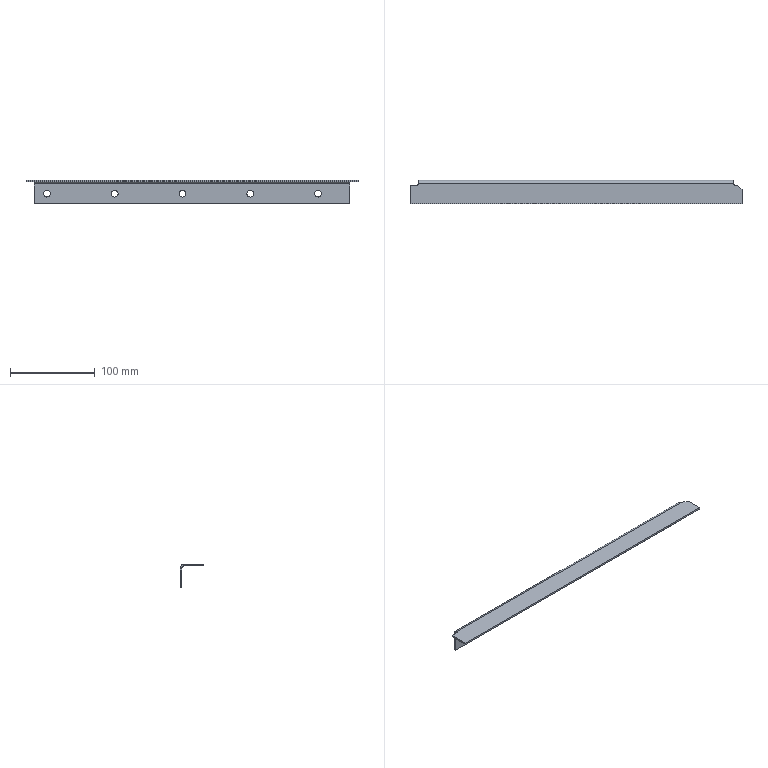Part | SolidWorks | features ICE 2, Chamfer 1, Fillet 1, FlatPattern 1, SMBaseFlange 1, SheetMetal 1 | 1 solid | 29 faces | box 391.9 x 28 x 28 mm | volume 39440 mm3 | plane 15 | cylinder 14 | commonest cylinder face diameters 8 x10 4 x2 5 x1 9 x1
STEP:
#1=CARTESIAN_POINT('',(-171.25,-2.,8.));
#2=VERTEX_POINT('',#1);
#3=CARTESIAN_POINT('',(-171.25,-2.,16.));
#4=VERTEX_POINT('',#3);
#5=CARTESIAN_POINT('',(-171.25,-2.,12.));
#6=DIRECTION('',(0.,1.,0.));
#7=DIRECTION('',(0.,0.,-1.));
#8=AXIS2_PLACEMENT_3D('',#5,#6,#7);
#9=CIRCLE('',#8,4.);
#10=EDGE_CURVE('',#2,#4,#9,.T.);
#11=ORIENTED_EDGE('',*,*,#10,.F.);
#12=CARTESIAN_POINT('',(-171.25,0.,8.));
#13=VERTEX_POINT('',#12);
#14=CARTESIAN_POINT('',(-171.25,-28.001,8.));
#15=DIRECTION('',(0.,1.,0.));
#16=VECTOR('',#15,1000.);
#17=LINE('',#14,#16);
#18=EDGE_CURVE('',#2,#13,#17,.T.);
#19=ORIENTED_EDGE('',*,*,#18,.T.);
#20=CARTESIAN_POINT('',(-171.25,0.,16.));
#21=VERTEX_POINT('',#20);
#22=CARTESIAN_POINT('',(-171.25,0.,12.));
#23=DIRECTION('',(0.,1.,0.));
#24=DIRECTION('',(0.,0.,1.));
#25=AXIS2_PLACEMENT_3D('',#22,#23,#24);
#26=CIRCLE('',#25,4.);
#27=EDGE_CURVE('',#13,#21,#26,.T.);
#28=ORIENTED_EDGE('',*,*,#27,.T.);
#29=CARTESIAN_POINT('',(-171.25,-28.001,16.));
#30=DIRECTION('',(0.,1.,0.));
#31=VECTOR('',#30,1000.);
#32=LINE('',#29,#31);
#33=EDGE_CURVE('',#4,#21,#32,.T.);
#34=ORIENTED_EDGE('',*,*,#33,.F.);
#35=EDGE_LOOP('',(#11,#19,#28,#34));
#36=FACE_OUTER_BOUND('',#35,.T.);
#37=CARTESIAN_POINT('',(-171.25,-28.001,12.));
#38=DIRECTION('',(0.,1.,0.));
#39=DIRECTION('',(0.,0.,1.));
#40=AXIS2_PLACEMENT_3D('',#37,#38,#39);
#41=CYLINDRICAL_SURFACE('',#40,4.);
#42=ADVANCED_FACE('',(#36),#41,.F.);
#43=CARTESIAN_POINT('',(-91.25,-2.,8.));
#44=VERTEX_POINT('',#43);
#45=CARTESIAN_POINT('',(-91.25,-2.,16.));
#46=VERTEX_POINT('',#45);
#47=CARTESIAN_POINT('',(-91.25,-2.,12.));
#48=DIRECTION('',(0.,1.,0.));
#49=DIRECTION('',(0.,0.,-1.));
#50=AXIS2_PLACEMENT_3D('',#47,#48,#49);
#51=CIRCLE('',#50,4.);
#52=EDGE_CURVE('',#44,#46,#51,.T.);
#53=ORIENTED_EDGE('',*,*,#52,.F.);
#54=CARTESIAN_POINT('',(-91.25,0.,8.));
#55=VERTEX_POINT('',#54);
#56=CARTESIAN_POINT('',(-91.25,-28.001,8.));
#57=DIRECTION('',(0.,1.,0.));
#58=VECTOR('',#57,1000.);
#59=LINE('',#56,#58);
#60=EDGE_CURVE('',#44,#55,#59,.T.);
#61=ORIENTED_EDGE('',*,*,#60,.T.);
#62=CARTESIAN_POINT('',(-91.25,0.,16.));
#63=VERTEX_POINT('',#62);
#64=CARTESIAN_POINT('',(-91.25,0.,12.));
#65=DIRECTION('',(0.,1.,0.));
#66=DIRECTION('',(0.,0.,1.));
#67=AXIS2_PLACEMENT_3D('',#64,#65,#66);
#68=CIRCLE('',#67,4.);
#69=EDGE_CURVE('',#55,#63,#68,.T.);
#70=ORIENTED_EDGE('',*,*,#69,.T.);
#71=CARTESIAN_POINT('',(-91.25,-28.001,16.));
#72=DIRECTION('',(0.,1.,0.));
#73=VECTOR('',#72,1000.);
#74=LINE('',#71,#73);
#75=EDGE_CURVE('',#46,#63,#74,.T.);
#76=ORIENTED_EDGE('',*,*,#75,.F.);
#77=EDGE_LOOP('',(#53,#61,#70,#76));
#78=FACE_OUTER_BOUND('',#77,.T.);
#79=CARTESIAN_POINT('',(-91.25,-28.001,12.));
#80=DIRECTION('',(0.,1.,0.));
#81=DIRECTION('',(0.,0.,1.));
#82=AXIS2_PLACEMENT_3D('',#79,#80,#81);
#83=CYLINDRICAL_SURFACE('',#82,4.);
#84=ADVANCED_FACE('',(#78),#83,.F.);
#85=CARTESIAN_POINT('',(-11.25,-2.,8.));
#86=VERTEX_POINT('',#85);
#87=CARTESIAN_POINT('',(-11.25,-2.,16.));
#88=VERTEX_POINT('',#87);
#89=CARTESIAN_POINT('',(-11.25,-2.,12.));
#90=DIRECTION('',(0.,1.,0.));
#91=DIRECTION('',(0.,0.,-1.));
#92=AXIS2_PLACEMENT_3D('',#89,#90,#91);
#93=CIRCLE('',#92,4.);
#94=EDGE_CURVE('',#86,#88,#93,.T.);
#95=ORIENTED_EDGE('',*,*,#94,.F.);
#96=CARTESIAN_POINT('',(-11.25,0.,8.));
#97=VERTEX_POINT('',#96);
#98=CARTESIAN_POINT('',(-11.25,-28.001,8.));
#99=DIRECTION('',(0.,1.,0.));
#100=VECTOR('',#99,1000.);
#101=LINE('',#98,#100);
#102=EDGE_CURVE('',#86,#97,#101,.T.);
#103=ORIENTED_EDGE('',*,*,#102,.T.);
#104=CARTESIAN_POINT('',(-11.25,0.,16.));
#105=VERTEX_POINT('',#104);
#106=CARTESIAN_POINT('',(-11.25,0.,12.));
#107=DIRECTION('',(0.,1.,0.));
#108=DIRECTION('',(0.,0.,1.));
#109=AXIS2_PLACEMENT_3D('',#106,#107,#108);
#110=CIRCLE('',#109,4.);
#111=EDGE_CURVE('',#97,#105,#110,.T.);
#112=ORIENTED_EDGE('',*,*,#111,.T.);
#113=CARTESIAN_POINT('',(-11.25,-28.001,16.));
#114=DIRECTION('',(0.,1.,0.));
#115=VECTOR('',#114,1000.);
#116=LINE('',#113,#115);
#117=EDGE_CURVE('',#88,#105,#116,.T.);
#118=ORIENTED_EDGE('',*,*,#117,.F.);
#119=EDGE_LOOP('',(#95,#103,#112,#118));
#120=FACE_OUTER_BOUND('',#119,.T.);
#121=CARTESIAN_POINT('',(-11.25,-28.001,12.));
#122=DIRECTION('',(0.,1.,0.));
#123=DIRECTION('',(0.,0.,1.));
#124=AXIS2_PLACEMENT_3D('',#121,#122,#123);
#125=CYLINDRICAL_SURFACE('',#124,4.);
#126=ADVANCED_FACE('',(#120),#125,.F.);
#127=CARTESIAN_POINT('',(68.75,-2.,8.));
#128=VERTEX_POINT('',#127);
#129=CARTESIAN_POINT('',(68.75,-2.,16.));
#130=VERTEX_POINT('',#129);
#131=CARTESIAN_POINT('',(68.75,-2.,12.));
#132=DIRECTION('',(0.,1.,0.));
#133=DIRECTION('',(0.,0.,-1.));
#134=AXIS2_PLACEMENT_3D('',#131,#132,#133);
#135=CIRCLE('',#134,4.);
#136=EDGE_CURVE('',#128,#130,#135,.T.);
#137=ORIENTED_EDGE('',*,*,#136,.F.);
#138=CARTESIAN_POINT('',(68.75,0.,8.));
#139=VERTEX_POINT('',#138);
#140=CARTESIAN_POINT('',(68.75,-28.001,8.));
#141=DIRECTION('',(0.,1.,0.));
#142=VECTOR('',#141,1000.);
#143=LINE('',#140,#142);
#144=EDGE_CURVE('',#128,#139,#143,.T.);
#145=ORIENTED_EDGE('',*,*,#144,.T.);
#146=CARTESIAN_POINT('',(68.75,0.,16.));
#147=VERTEX_POINT('',#146);
#148=CARTESIAN_POINT('',(68.75,0.,12.));
#149=DIRECTION('',(0.,1.,0.));
#150=DIRECTION('',(0.,0.,1.));
#151=AXIS2_PLACEMENT_3D('',#148,#149,#150);
#152=CIRCLE('',#151,4.);
#153=EDGE_CURVE('',#139,#147,#152,.T.);
#154=ORIENTED_EDGE('',*,*,#153,.T.);
#155=CARTESIAN_POINT('',(68.75,-28.001,16.));
#156=DIRECTION('',(0.,1.,0.));
#157=VECTOR('',#156,1000.);
#158=LINE('',#155,#157);
#159=EDGE_CURVE('',#130,#147,#158,.T.);
#160=ORIENTED_EDGE('',*,*,#159,.F.);
#161=EDGE_LOOP('',(#137,#145,#154,#160));
#162=FACE_OUTER_BOUND('',#161,.T.);
#163=CARTESIAN_POINT('',(68.75,-28.001,12.));
#164=DIRECTION('',(0.,1.,0.));
#165=DIRECTION('',(0.,0.,1.));
#166=AXIS2_PLACEMENT_3D('',#163,#164,#165);
#167=CYLINDRICAL_SURFACE('',#166,4.);
#168=ADVANCED_FACE('',(#162),#167,.F.);
#169=CARTESIAN_POINT('',(148.75,-2.,8.));
#170=VERTEX_POINT('',#169);
#171=CARTESIAN_POINT('',(148.75,-2.,16.));
#172=VERTEX_POINT('',#171);
#173=CARTESIAN_POINT('',(148.75,-2.,12.));
#174=DIRECTION('',(0.,1.,0.));
#175=DIRECTION('',(0.,0.,-1.));
#176=AXIS2_PLACEMENT_3D('',#173,#174,#175);
#177=CIRCLE('',#176,4.);
#178=EDGE_CURVE('',#170,#172,#177,.T.);
#179=ORIENTED_EDGE('',*,*,#178,.F.);
#180=CARTESIAN_POINT('',(148.75,0.,8.));
#181=VERTEX_POINT('',#180);
#182=CARTESIAN_POINT('',(148.75,-28.001,8.));
#183=DIRECTION('',(0.,1.,0.));
#184=VECTOR('',#183,1000.);
#185=LINE('',#182,#184);
#186=EDGE_CURVE('',#170,#181,#185,.T.);
#187=ORIENTED_EDGE('',*,*,#186,.T.);
#188=CARTESIAN_POINT('',(148.75,0.,16.));
#189=VERTEX_POINT('',#188);
#190=CARTESIAN_POINT('',(148.75,0.,12.));
#191=DIRECTION('',(0.,1.,0.));
#192=DIRECTION('',(0.,0.,1.));
#193=AXIS2_PLACEMENT_3D('',#190,#191,#192);
#194=CIRCLE('',#193,4.);
#195=EDGE_CURVE('',#181,#189,#194,.T.);
#196=ORIENTED_EDGE('',*,*,#195,.T.);
#197=CARTESIAN_POINT('',(148.75,-28.001,16.));
#198=DIRECTION('',(0.,1.,0.));
#199=VECTOR('',#198,1000.);
#200=LINE('',#197,#199);
#201=EDGE_CURVE('',#172,#189,#200,.T.);
#202=ORIENTED_EDGE('',*,*,#201,.F.);
#203=EDGE_LOOP('',(#179,#187,#196,#202));
#204=FACE_OUTER_BOUND('',#203,.T.);
#205=CARTESIAN_POINT('',(148.75,-28.001,12.));
#206=DIRECTION('',(0.,1.,0.));
#207=DIRECTION('',(0.,0.,1.));
#208=AXIS2_PLACEMENT_3D('',#205,#206,#207);
#209=CYLINDRICAL_SURFACE('',#208,4.);
#210=ADVANCED_FACE('',(#204),#209,.F.);
#211=CARTESIAN_POINT('',(-186.25,-2.,0.));
#212=VERTEX_POINT('',#211);
#213=CARTESIAN_POINT('',(-186.25,-2.,23.5));
#214=VERTEX_POINT('',#213);
#215=CARTESIAN_POINT('',(-186.25,-2.,0.));
#216=DIRECTION('',(0.,0.,1.));
#217=VECTOR('',#216,1000.);
#218=LINE('',#215,#217);
#219=EDGE_CURVE('',#212,#214,#218,.T.);
#220=ORIENTED_EDGE('',*,*,#219,.T.);
#221=CARTESIAN_POINT('',(-186.25,0.,23.5));
#222=VERTEX_POINT('',#221);
#223=CARTESIAN_POINT('',(-186.25,-2.,23.5));
#224=DIRECTION('',(0.,1.,0.));
#225=VECTOR('',#224,1000.);
#226=LINE('',#223,#225);
#227=EDGE_CURVE('',#214,#222,#226,.T.);
#228=ORIENTED_EDGE('',*,*,#227,.T.);
#229=CARTESIAN_POINT('',(-186.25,0.,0.));
#230=VERTEX_POINT('',#229);
#231=CARTESIAN_POINT('',(-186.25,0.,0.));
#232=DIRECTION('',(0.,0.,1.));
#233=VECTOR('',#232,1000.);
#234=LINE('',#231,#233);
#235=EDGE_CURVE('',#230,#222,#234,.T.);
#236=ORIENTED_EDGE('',*,*,#235,.F.);
#237=CARTESIAN_POINT('',(-186.25,0.,0.));
#238=DIRECTION('',(0.,1.,0.));
#239=VECTOR('',#238,1000.);
#240=LINE('',#237,#239);
#241=EDGE_CURVE('',#212,#230,#240,.T.);
#242=ORIENTED_EDGE('',*,*,#241,.F.);
#243=EDGE_LOOP('',(#220,#228,#236,#242));
#244=FACE_OUTER_BOUND('',#243,.T.);
#245=CARTESIAN_POINT('',(-186.25,0.,0.));
#246=DIRECTION('',(1.,0.,0.));
#247=DIRECTION('',(0.,0.,-1.));
#248=AXIS2_PLACEMENT_3D('',#245,#246,#247);
#249=PLANE('',#248);
#250=ADVANCED_FACE('',(#244),#249,.F.);
#251=CARTESIAN_POINT('',(186.25,0.,0.));
#252=VERTEX_POINT('',#251);
#253=CARTESIAN_POINT('',(186.25,0.,23.5));
#254=VERTEX_POINT('',#253);
#255=CARTESIAN_POINT('',(186.25,0.,0.));
#256=DIRECTION('',(0.,0.,1.));
#257=VECTOR('',#256,1000.);
#258=LINE('',#255,#257);
#259=EDGE_CURVE('',#252,#254,#258,.T.);
#260=ORIENTED_EDGE('',*,*,#259,.T.);
#261=CARTESIAN_POINT('',(186.25,-2.,23.5));
#262=VERTEX_POINT('',#261);
#263=CARTESIAN_POINT('',(186.25,0.,23.5));
#264=DIRECTION('',(0.,-1.,0.));
#265=VECTOR('',#264,1000.);
#266=LINE('',#263,#265);
#267=EDGE_CURVE('',#254,#262,#266,.T.);
#268=ORIENTED_EDGE('',*,*,#267,.T.);
#269=CARTESIAN_POINT('',(186.25,-2.,0.));
#270=VERTEX_POINT('',#269);
#271=CARTESIAN_POINT('',(186.25,-2.,0.));
#272=DIRECTION('',(0.,0.,-1.));
#273=VECTOR('',#272,1000.);
#274=LINE('',#271,#273);
#275=EDGE_CURVE('',#262,#270,#274,.T.);
#276=ORIENTED_EDGE('',*,*,#275,.T.);
#277=CARTESIAN_POINT('',(186.25,0.,0.));
#278=DIRECTION('',(0.,-1.,0.));
#279=VECTOR('',#278,1000.);
#280=LINE('',#277,#279);
#281=EDGE_CURVE('',#252,#270,#280,.T.);
#282=ORIENTED_EDGE('',*,*,#281,.F.);
#283=EDGE_LOOP('',(#260,#268,#276,#282));
#284=FACE_OUTER_BOUND('',#283,.T.);
#285=CARTESIAN_POINT('',(186.25,0.,0.));
#286=DIRECTION('',(-1.,0.,0.));
#287=DIRECTION('',(0.,0.,1.));
#288=AXIS2_PLACEMENT_3D('',#285,#286,#287);
#289=PLANE('',#288);
#290=ADVANCED_FACE('',(#284),#289,.F.);
#291=CARTESIAN_POINT('',(-195.95,-6.,26.));
#292=VERTEX_POINT('',#291);
#293=CARTESIAN_POINT('',(-195.95,-6.,28.));
#294=VERTEX_POINT('',#293);
#295=CARTESIAN_POINT('',(-195.95,-6.,0.));
#296=DIRECTION('',(0.,0.,1.));
#297=VECTOR('',#296,1000.);
#298=LINE('',#295,#297);
#299=EDGE_CURVE('',#292,#294,#298,.T.);
#300=ORIENTED_EDGE('',*,*,#299,.F.);
#301=CARTESIAN_POINT('',(-195.95,-28.,26.));
#302=VERTEX_POINT('',#301);
#303=CARTESIAN_POINT('',(-195.95,0.,26.));
#304=DIRECTION('',(0.,-1.,0.));
#305=VECTOR('',#304,1000.);
#306=LINE('',#303,#305);
#307=EDGE_CURVE('',#292,#302,#306,.T.);
#308=ORIENTED_EDGE('',*,*,#307,.T.);
#309=CARTESIAN_POINT('',(-195.95,-28.,28.));
#310=VERTEX_POINT('',#309);
#311=CARTESIAN_POINT('',(-195.95,-28.,26.));
#312=DIRECTION('',(0.,0.,1.));
#313=VECTOR('',#312,1000.);
#314=LINE('',#311,#313);
#315=EDGE_CURVE('',#302,#310,#314,.T.);
#316=ORIENTED_EDGE('',*,*,#315,.T.);
#317=CARTESIAN_POINT('',(-195.95,0.,28.));
#318=DIRECTION('',(0.,-1.,0.));
#319=VECTOR('',#318,1000.);
#320=LINE('',#317,#319);
#321=EDGE_CURVE('',#294,#310,#320,.T.);
#322=ORIENTED_EDGE('',*,*,#321,.F.);
#323=EDGE_LOOP('',(#300,#308,#316,#322));
#324=FACE_OUTER_BOUND('',#323,.T.);
#325=CARTESIAN_POINT('',(-195.95,-2.,23.5));
#326=DIRECTION('',(-1.,0.,0.));
#327=DIRECTION('',(0.,0.,1.));
#328=AXIS2_PLACEMENT_3D('',#325,#326,#327);
#329=PLANE('',#328);
#330=ADVANCED_FACE('',(#324),#329,.T.);
#331=CARTESIAN_POINT('',(195.95,-11.,28.));
#332=VERTEX_POINT('',#331);
#333=CARTESIAN_POINT('',(195.95,-28.,28.));
#334=VERTEX_POINT('',#333);
#335=CARTESIAN_POINT('',(195.95,0.,28.));
#336=DIRECTION('',(0.,-1.,0.));
#337=VECTOR('',#336,1000.);
#338=LINE('',#335,#337);
#339=EDGE_CURVE('',#332,#334,#338,.T.);
#340=ORIENTED_EDGE('',*,*,#339,.F.);
#341=CARTESIAN_POINT('',(190.95,-6.,28.));
#342=VERTEX_POINT('',#341);
#343=CARTESIAN_POINT('',(190.95,-6.,28.));
#344=DIRECTION('',(-0.7071,0.7071,0.));
#345=VECTOR('',#344,1000.);
#346=LINE('',#343,#345);
#347=EDGE_CURVE('',#332,#342,#346,.T.);
#348=ORIENTED_EDGE('',*,*,#347,.T.);
#349=CARTESIAN_POINT('',(188.25,-6.,28.));
#350=VERTEX_POINT('',#349);
#351=CARTESIAN_POINT('',(195.95,-6.,28.));
#352=DIRECTION('',(1.,0.,0.));
#353=VECTOR('',#352,1000.);
#354=LINE('',#351,#353);
#355=EDGE_CURVE('',#350,#342,#354,.T.);
#356=ORIENTED_EDGE('',*,*,#355,.F.);
#357=CARTESIAN_POINT('',(186.314,-4.5,28.));
#358=VERTEX_POINT('',#357);
#359=CARTESIAN_POINT('',(188.25,-4.,28.));
#360=DIRECTION('',(0.,0.,-1.));
#361=DIRECTION('',(0.,1.,0.));
#362=AXIS2_PLACEMENT_3D('',#359,#360,#361);
#363=CIRCLE('',#362,2.);
#364=EDGE_CURVE('',#350,#358,#363,.T.);
#365=ORIENTED_EDGE('',*,*,#364,.T.);
#366=CARTESIAN_POINT('',(-186.314,-4.5,28.));
#367=VERTEX_POINT('',#366);
#368=CARTESIAN_POINT('',(195.95,-4.5,28.));
#369=DIRECTION('',(-1.,0.,0.));
#370=VECTOR('',#369,1000.);
#371=LINE('',#368,#370);
#372=EDGE_CURVE('',#358,#367,#371,.T.);
#373=ORIENTED_EDGE('',*,*,#372,.T.);
#374=CARTESIAN_POINT('',(-188.25,-6.,28.));
#375=VERTEX_POINT('',#374);
#376=CARTESIAN_POINT('',(-188.25,-4.,28.));
#377=DIRECTION('',(0.,0.,-1.));
#378=DIRECTION('',(0.,1.,0.));
#379=AXIS2_PLACEMENT_3D('',#376,#377,#378);
#380=CIRCLE('',#379,2.);
#381=EDGE_CURVE('',#367,#375,#380,.T.);
#382=ORIENTED_EDGE('',*,*,#381,.T.);
#383=CARTESIAN_POINT('',(-195.95,-6.,28.));
#384=DIRECTION('',(1.,0.,0.));
#385=VECTOR('',#384,1000.);
#386=LINE('',#383,#385);
#387=EDGE_CURVE('',#294,#375,#386,.T.);
#388=ORIENTED_EDGE('',*,*,#387,.F.);
#389=ORIENTED_EDGE('',*,*,#321,.T.);
#390=CARTESIAN_POINT('',(195.95,-28.,28.));
#391=DIRECTION('',(-1.,0.,0.));
#392=VECTOR('',#391,1000.);
#393=LINE('',#390,#392);
#394=EDGE_CURVE('',#334,#310,#393,.T.);
#395=ORIENTED_EDGE('',*,*,#394,.F.);
#396=EDGE_LOOP('',(#340,#348,#356,#365,#373,#382,#388,#389,#395));
#397=FACE_OUTER_BOUND('',#396,.T.);
#398=CARTESIAN_POINT('',(195.95,0.,28.));
#399=DIRECTION('',(0.,0.,-1.));
#400=DIRECTION('',(0.,1.,0.));
#401=AXIS2_PLACEMENT_3D('',#398,#399,#400);
#402=PLANE('',#401);
#403=ADVANCED_FACE('',(#397),#402,.F.);
#404=ORIENTED_EDGE('',*,*,#315,.F.);
#405=CARTESIAN_POINT('',(195.95,-28.,26.));
#406=VERTEX_POINT('',#405);
#407=CARTESIAN_POINT('',(195.95,-28.,26.));
#408=DIRECTION('',(-1.,0.,0.));
#409=VECTOR('',#408,1000.);
#410=LINE('',#407,#409);
#411=EDGE_CURVE('',#406,#302,#410,.T.);
#412=ORIENTED_EDGE('',*,*,#411,.F.);
#413=CARTESIAN_POINT('',(195.95,-28.,26.));
#414=DIRECTION('',(0.,0.,1.));
#415=VECTOR('',#414,1000.);
#416=LINE('',#413,#415);
#417=EDGE_CURVE('',#406,#334,#416,.T.);
#418=ORIENTED_EDGE('',*,*,#417,.T.);
#419=ORIENTED_EDGE('',*,*,#394,.T.);
#420=EDGE_LOOP('',(#404,#412,#418,#419));
#421=FACE_OUTER_BOUND('',#420,.T.);
#422=CARTESIAN_POINT('',(195.95,-28.,26.));
#423=DIRECTION('',(0.,-1.,0.));
#424=DIRECTION('',(0.,0.,-1.));
#425=AXIS2_PLACEMENT_3D('',#422,#423,#424);
#426=PLANE('',#425);
#427=ADVANCED_FACE('',(#421),#426,.T.);
#428=CARTESIAN_POINT('',(190.95,-6.,26.));
#429=VERTEX_POINT('',#428);
#430=CARTESIAN_POINT('',(188.25,-6.,26.));
#431=VERTEX_POINT('',#430);
#432=CARTESIAN_POINT('',(195.95,-6.,26.));
#433=DIRECTION('',(-1.,0.,0.));
#434=VECTOR('',#433,1000.);
#435=LINE('',#432,#434);
#436=EDGE_CURVE('',#429,#431,#435,.T.);
#437=ORIENTED_EDGE('',*,*,#436,.F.);
#438=CARTESIAN_POINT('',(195.95,-11.,26.));
#439=VERTEX_POINT('',#438);
#440=CARTESIAN_POINT('',(190.45,-5.5,26.));
#441=DIRECTION('',(0.7071,-0.7071,0.));
#442=VECTOR('',#441,1000.);
#443=LINE('',#440,#442);
#444=EDGE_CURVE('',#429,#439,#443,.T.);
#445=ORIENTED_EDGE('',*,*,#444,.T.);
#446=CARTESIAN_POINT('',(195.95,0.,26.));
#447=DIRECTION('',(0.,-1.,0.));
#448=VECTOR('',#447,1000.);
#449=LINE('',#446,#448);
#450=EDGE_CURVE('',#439,#406,#449,.T.);
#451=ORIENTED_EDGE('',*,*,#450,.T.);
#452=ORIENTED_EDGE('',*,*,#411,.T.);
#453=ORIENTED_EDGE('',*,*,#307,.F.);
#454=CARTESIAN_POINT('',(-188.25,-6.,26.));
#455=VERTEX_POINT('',#454);
#456=CARTESIAN_POINT('',(195.95,-6.,26.));
#457=DIRECTION('',(-1.,0.,0.));
#458=VECTOR('',#457,1000.);
#459=LINE('',#456,#458);
#460=EDGE_CURVE('',#455,#292,#459,.T.);
#461=ORIENTED_EDGE('',*,*,#460,.F.);
#462=CARTESIAN_POINT('',(-186.314,-4.5,26.));
#463=VERTEX_POINT('',#462);
#464=CARTESIAN_POINT('',(-188.25,-4.,26.));
#465=DIRECTION('',(0.,0.,1.));
#466=DIRECTION('',(0.,1.,0.));
#467=AXIS2_PLACEMENT_3D('',#464,#465,#466);
#468=CIRCLE('',#467,2.);
#469=EDGE_CURVE('',#455,#463,#468,.T.);
#470=ORIENTED_EDGE('',*,*,#469,.T.);
#471=CARTESIAN_POINT('',(186.314,-4.5,26.));
#472=VERTEX_POINT('',#471);
#473=CARTESIAN_POINT('',(195.95,-4.5,26.));
#474=DIRECTION('',(-1.,0.,0.));
#475=VECTOR('',#474,1000.);
#476=LINE('',#473,#475);
#477=EDGE_CURVE('',#472,#463,#476,.T.);
#478=ORIENTED_EDGE('',*,*,#477,.F.);
#479=CARTESIAN_POINT('',(188.25,-4.,26.));
#480=DIRECTION('',(0.,0.,1.));
#481=DIRECTION('',(0.,1.,0.));
#482=AXIS2_PLACEMENT_3D('',#479,#480,#481);
#483=CIRCLE('',#482,2.);
#484=EDGE_CURVE('',#472,#431,#483,.T.);
#485=ORIENTED_EDGE('',*,*,#484,.T.);
#486=EDGE_LOOP('',(#437,#445,#451,#452,#453,#461,#470,#478,#485));
#487=FACE_OUTER_BOUND('',#486,.T.);
#488=CARTESIAN_POINT('',(195.95,0.,26.));
#489=DIRECTION('',(0.,0.,-1.));
#490=DIRECTION('',(0.,1.,0.));
#491=AXIS2_PLACEMENT_3D('',#488,#489,#490);
#492=PLANE('',#491);
#493=ADVANCED_FACE('',(#487),#492,.T.);
#494=CARTESIAN_POINT('',(-186.25,-4.,25.949));
#495=VERTEX_POINT('',#494);
#496=CARTESIAN_POINT('',(-186.25,-4.5,23.5));
#497=DIRECTION('',(1.,0.,0.));
#498=DIRECTION('',(0.,0.,-1.));
#499=AXIS2_PLACEMENT_3D('',#496,#497,#498);
#500=CIRCLE('',#499,2.5);
#501=EDGE_CURVE('',#214,#495,#500,.T.);
#502=ORIENTED_EDGE('',*,*,#501,.F.);
#503=CARTESIAN_POINT('',(195.95,-2.,23.5));
#504=DIRECTION('',(-1.,0.,0.));
#505=VECTOR('',#504,1000.);
#506=LINE('',#503,#505);
#507=EDGE_CURVE('',#262,#214,#506,.T.);
#508=ORIENTED_EDGE('',*,*,#507,.F.);
#509=CARTESIAN_POINT('',(186.25,-4.,25.949));
#510=VERTEX_POINT('',#509);
#511=CARTESIAN_POINT('',(186.25,-4.5,23.5));
#512=DIRECTION('',(-1.,0.,0.));
#513=DIRECTION('',(0.,0.,1.));
#514=AXIS2_PLACEMENT_3D('',#511,#512,#513);
#515=CIRCLE('',#514,2.5);
#516=EDGE_CURVE('',#510,#262,#515,.T.);
#517=ORIENTED_EDGE('',*,*,#516,.F.);
#518=CARTESIAN_POINT('',(186.25,-4.,25.949));
#519=CARTESIAN_POINT('',(186.25,-4.168,25.984));
#520=CARTESIAN_POINT('',(186.271,-4.334,26.));
#521=CARTESIAN_POINT('',(186.314,-4.5,26.));
#522=B_SPLINE_CURVE_WITH_KNOTS('',3,(#518,#519,#520,#521),.UNSPECIFIED.,.F.,.F.,(4,4),(0.,0.0005065),.UNSPECIFIED.);
#523=EDGE_CURVE('',#510,#472,#522,.T.);
#524=ORIENTED_EDGE('',*,*,#523,.T.);
#525=ORIENTED_EDGE('',*,*,#477,.T.);
#526=CARTESIAN_POINT('',(-186.314,-4.5,26.));
#527=CARTESIAN_POINT('',(-186.271,-4.334,26.));
#528=CARTESIAN_POINT('',(-186.25,-4.168,25.984));
#529=CARTESIAN_POINT('',(-186.25,-4.,25.949));
#530=B_SPLINE_CURVE_WITH_KNOTS('',3,(#526,#527,#528,#529),.UNSPECIFIED.,.F.,.F.,(4,4),(0.,0.0005065),.UNSPECIFIED.);
#531=EDGE_CURVE('',#463,#495,#530,.T.);
#532=ORIENTED_EDGE('',*,*,#531,.T.);
#533=EDGE_LOOP('',(#502,#508,#517,#524,#525,#532));
#534=FACE_OUTER_BOUND('',#533,.T.);
#535=CARTESIAN_POINT('',(195.95,-4.5,23.5));
#536=DIRECTION('',(-1.,0.,0.));
#537=DIRECTION('',(0.,0.,1.));
#538=AXIS2_PLACEMENT_3D('',#535,#536,#537);
#539=CYLINDRICAL_SURFACE('',#538,2.5);
#540=ADVANCED_FACE('',(#534),#539,.F.);
#541=CARTESIAN_POINT('',(-171.25,-2.,12.));
#542=DIRECTION('',(0.,1.,0.));
#543=DIRECTION('',(0.,0.,-1.));
#544=AXIS2_PLACEMENT_3D('',#541,#542,#543);
#545=CIRCLE('',#544,4.);
#546=EDGE_CURVE('',#4,#2,#545,.T.);
#547=ORIENTED_EDGE('',*,*,#546,.T.);
#548=ORIENTED_EDGE('',*,*,#10,.T.);
#549=EDGE_LOOP('',(#547,#548));
#550=FACE_BOUND('',#549,.T.);
#551=CARTESIAN_POINT('',(-91.25,-2.,12.));
#552=DIRECTION('',(0.,1.,0.));
#553=DIRECTION('',(0.,0.,-1.));
#554=AXIS2_PLACEMENT_3D('',#551,#552,#553);
#555=CIRCLE('',#554,4.);
#556=EDGE_CURVE('',#46,#44,#555,.T.);
#557=ORIENTED_EDGE('',*,*,#556,.T.);
#558=ORIENTED_EDGE('',*,*,#52,.T.);
#559=EDGE_LOOP('',(#557,#558));
#560=FACE_BOUND('',#559,.T.);
#561=CARTESIAN_POINT('',(-11.25,-2.,12.));
#562=DIRECTION('',(0.,1.,0.));
#563=DIRECTION('',(0.,0.,-1.));
#564=AXIS2_PLACEMENT_3D('',#561,#562,#563);
#565=CIRCLE('',#564,4.);
#566=EDGE_CURVE('',#88,#86,#565,.T.);
#567=ORIENTED_EDGE('',*,*,#566,.T.);
#568=ORIENTED_EDGE('',*,*,#94,.T.);
#569=EDGE_LOOP('',(#567,#568));
#570=FACE_BOUND('',#569,.T.);
#571=CARTESIAN_POINT('',(68.75,-2.,12.));
#572=DIRECTION('',(0.,1.,0.));
#573=DIRECTION('',(0.,0.,-1.));
#574=AXIS2_PLACEMENT_3D('',#571,#572,#573);
#575=CIRCLE('',#574,4.);
#576=EDGE_CURVE('',#130,#128,#575,.T.);
#577=ORIENTED_EDGE('',*,*,#576,.T.);
#578=ORIENTED_EDGE('',*,*,#136,.T.);
#579=EDGE_LOOP('',(#577,#578));
#580=FACE_BOUND('',#579,.T.);
#581=CARTESIAN_POINT('',(148.75,-2.,12.));
#582=DIRECTION('',(0.,1.,0.));
#583=DIRECTION('',(0.,0.,-1.));
#584=AXIS2_PLACEMENT_3D('',#581,#582,#583);
#585=CIRCLE('',#584,4.);
#586=EDGE_CURVE('',#172,#170,#585,.T.);
#587=ORIENTED_EDGE('',*,*,#586,.T.);
#588=ORIENTED_EDGE('',*,*,#178,.T.);
#589=EDGE_LOOP('',(#587,#588));
#590=FACE_BOUND('',#589,.T.);
#591=ORIENTED_EDGE('',*,*,#219,.F.);
#592=CARTESIAN_POINT('',(195.95,-2.,0.));
#593=DIRECTION('',(-1.,0.,0.));
#594=VECTOR('',#593,1000.);
#595=LINE('',#592,#594);
#596=EDGE_CURVE('',#270,#212,#595,.T.);
#597=ORIENTED_EDGE('',*,*,#596,.F.);
#598=ORIENTED_EDGE('',*,*,#275,.F.);
#599=ORIENTED_EDGE('',*,*,#507,.T.);
#600=EDGE_LOOP('',(#591,#597,#598,#599));
#601=FACE_OUTER_BOUND('',#600,.T.);
#602=CARTESIAN_POINT('',(195.95,-2.,0.));
#603=DIRECTION('',(0.,-1.,0.));
#604=DIRECTION('',(0.,0.,-1.));
#605=AXIS2_PLACEMENT_3D('',#602,#603,#604);
#606=PLANE('',#605);
#607=ADVANCED_FACE('',(#550,#560,#570,#580,#590,#601),#606,.T.);
#608=ORIENTED_EDGE('',*,*,#241,.T.);
#609=CARTESIAN_POINT('',(195.95,0.,0.));
#610=DIRECTION('',(-1.,0.,0.));
#611=VECTOR('',#610,1000.);
#612=LINE('',#609,#611);
#613=EDGE_CURVE('',#252,#230,#612,.T.);
#614=ORIENTED_EDGE('',*,*,#613,.F.);
#615=ORIENTED_EDGE('',*,*,#281,.T.);
#616=ORIENTED_EDGE('',*,*,#596,.T.);
#617=EDGE_LOOP('',(#608,#614,#615,#616));
#618=FACE_OUTER_BOUND('',#617,.T.);
#619=CARTESIAN_POINT('',(195.95,0.,0.));
#620=DIRECTION('',(0.,0.,-1.));
#621=DIRECTION('',(-1.,0.,0.));
#622=AXIS2_PLACEMENT_3D('',#619,#620,#621);
#623=PLANE('',#622);
#624=ADVANCED_FACE('',(#618),#623,.T.);
#625=CARTESIAN_POINT('',(-171.25,0.,12.));
#626=DIRECTION('',(0.,1.,0.));
#627=DIRECTION('',(0.,0.,1.));
#628=AXIS2_PLACEMENT_3D('',#625,#626,#627);
#629=CIRCLE('',#628,4.);
#630=EDGE_CURVE('',#21,#13,#629,.T.);
#631=ORIENTED_EDGE('',*,*,#630,.F.);
#632=ORIENTED_EDGE('',*,*,#27,.F.);
#633=EDGE_LOOP('',(#631,#632));
#634=FACE_BOUND('',#633,.T.);
#635=CARTESIAN_POINT('',(-91.25,0.,12.));
#636=DIRECTION('',(0.,1.,0.));
#637=DIRECTION('',(0.,0.,1.));
#638=AXIS2_PLACEMENT_3D('',#635,#636,#637);
#639=CIRCLE('',#638,4.);
#640=EDGE_CURVE('',#63,#55,#639,.T.);
#641=ORIENTED_EDGE('',*,*,#640,.F.);
#642=ORIENTED_EDGE('',*,*,#69,.F.);
#643=EDGE_LOOP('',(#641,#642));
#644=FACE_BOUND('',#643,.T.);
#645=CARTESIAN_POINT('',(-11.25,0.,12.));
#646=DIRECTION('',(0.,1.,0.));
#647=DIRECTION('',(0.,0.,1.));
#648=AXIS2_PLACEMENT_3D('',#645,#646,#647);
#649=CIRCLE('',#648,4.);
#650=EDGE_CURVE('',#105,#97,#649,.T.);
#651=ORIENTED_EDGE('',*,*,#650,.F.);
#652=ORIENTED_EDGE('',*,*,#111,.F.);
#653=EDGE_LOOP('',(#651,#652));
#654=FACE_BOUND('',#653,.T.);
#655=CARTESIAN_POINT('',(68.75,0.,12.));
#656=DIRECTION('',(0.,1.,0.));
#657=DIRECTION('',(0.,0.,1.));
#658=AXIS2_PLACEMENT_3D('',#655,#656,#657);
#659=CIRCLE('',#658,4.);
#660=EDGE_CURVE('',#147,#139,#659,.T.);
#661=ORIENTED_EDGE('',*,*,#660,.F.);
#662=ORIENTED_EDGE('',*,*,#153,.F.);
#663=EDGE_LOOP('',(#661,#662));
#664=FACE_BOUND('',#663,.T.);
#665=CARTESIAN_POINT('',(148.75,0.,12.));
#666=DIRECTION('',(0.,1.,0.));
#667=DIRECTION('',(0.,0.,1.));
#668=AXIS2_PLACEMENT_3D('',#665,#666,#667);
#669=CIRCLE('',#668,4.);
#670=EDGE_CURVE('',#189,#181,#669,.T.);
#671=ORIENTED_EDGE('',*,*,#670,.F.);
#672=ORIENTED_EDGE('',*,*,#195,.F.);
#673=EDGE_LOOP('',(#671,#672));
#674=FACE_BOUND('',#673,.T.);
#675=ORIENTED_EDGE('',*,*,#613,.T.);
#676=ORIENTED_EDGE('',*,*,#235,.T.);
#677=CARTESIAN_POINT('',(195.95,0.,23.5));
#678=DIRECTION('',(-1.,0.,0.));
#679=VECTOR('',#678,1000.);
#680=LINE('',#677,#679);
#681=EDGE_CURVE('',#254,#222,#680,.T.);
#682=ORIENTED_EDGE('',*,*,#681,.F.);
#683=ORIENTED_EDGE('',*,*,#259,.F.);
#684=EDGE_LOOP('',(#675,#676,#682,#683));
#685=FACE_OUTER_BOUND('',#684,.T.);
#686=CARTESIAN_POINT('',(195.95,0.,0.));
#687=DIRECTION('',(0.,-1.,0.));
#688=DIRECTION('',(0.,0.,-1.));
#689=AXIS2_PLACEMENT_3D('',#686,#687,#688);
#690=PLANE('',#689);
#691=ADVANCED_FACE('',(#634,#644,#654,#664,#674,#685),#690,.F.);
#692=ORIENTED_EDGE('',*,*,#681,.T.);
#693=CARTESIAN_POINT('',(-186.25,-4.,27.972));
#694=VERTEX_POINT('',#693);
#695=CARTESIAN_POINT('',(-186.25,-4.5,23.5));
#696=DIRECTION('',(1.,0.,0.));
#697=DIRECTION('',(0.,0.,-1.));
#698=AXIS2_PLACEMENT_3D('',#695,#696,#697);
#699=CIRCLE('',#698,4.5);
#700=EDGE_CURVE('',#222,#694,#699,.T.);
#701=ORIENTED_EDGE('',*,*,#700,.T.);
#702=CARTESIAN_POINT('',(-186.25,-4.,27.972));
#703=CARTESIAN_POINT('',(-186.25,-4.169,27.991));
#704=CARTESIAN_POINT('',(-186.271,-4.336,28.));
#705=CARTESIAN_POINT('',(-186.314,-4.5,28.));
#706=B_SPLINE_CURVE_WITH_KNOTS('',3,(#702,#703,#704,#705),.UNSPECIFIED.,.F.,.F.,(4,4),(0.,0.0005048),.UNSPECIFIED.);
#707=EDGE_CURVE('',#694,#367,#706,.T.);
#708=ORIENTED_EDGE('',*,*,#707,.T.);
#709=ORIENTED_EDGE('',*,*,#372,.F.);
#710=CARTESIAN_POINT('',(186.25,-4.,27.972));
#711=VERTEX_POINT('',#710);
#712=CARTESIAN_POINT('',(186.314,-4.5,28.));
#713=CARTESIAN_POINT('',(186.271,-4.336,28.));
#714=CARTESIAN_POINT('',(186.25,-4.169,27.991));
#715=CARTESIAN_POINT('',(186.25,-4.,27.972));
#716=B_SPLINE_CURVE_WITH_KNOTS('',3,(#712,#713,#714,#715),.UNSPECIFIED.,.F.,.F.,(4,4),(0.,0.0005048),.UNSPECIFIED.);
#717=EDGE_CURVE('',#358,#711,#716,.T.);
#718=ORIENTED_EDGE('',*,*,#717,.T.);
#719=CARTESIAN_POINT('',(186.25,-4.5,23.5));
#720=DIRECTION('',(-1.,0.,0.));
#721=DIRECTION('',(0.,0.,1.));
#722=AXIS2_PLACEMENT_3D('',#719,#720,#721);
#723=CIRCLE('',#722,4.5);
#724=EDGE_CURVE('',#711,#254,#723,.T.);
#725=ORIENTED_EDGE('',*,*,#724,.T.);
#726=EDGE_LOOP('',(#692,#701,#708,#709,#718,#725));
#727=FACE_OUTER_BOUND('',#726,.T.);
#728=CARTESIAN_POINT('',(195.95,-4.5,23.5));
#729=DIRECTION('',(-1.,0.,0.));
#730=DIRECTION('',(0.,0.,1.));
#731=AXIS2_PLACEMENT_3D('',#728,#729,#730);
#732=CYLINDRICAL_SURFACE('',#731,4.5);
#733=ADVANCED_FACE('',(#727),#732,.T.);
#734=ORIENTED_EDGE('',*,*,#450,.F.);
#735=CARTESIAN_POINT('',(195.95,-11.,28.));
#736=DIRECTION('',(0.,0.,1.));
#737=VECTOR('',#736,1000.);
#738=LINE('',#735,#737);
#739=EDGE_CURVE('',#439,#332,#738,.T.);
#740=ORIENTED_EDGE('',*,*,#739,.T.);
#741=ORIENTED_EDGE('',*,*,#339,.T.);
#742=ORIENTED_EDGE('',*,*,#417,.F.);
#743=EDGE_LOOP('',(#734,#740,#741,#742));
#744=FACE_OUTER_BOUND('',#743,.T.);
#745=CARTESIAN_POINT('',(195.95,-4.5,23.5));
#746=DIRECTION('',(1.,0.,0.));
#747=DIRECTION('',(0.,0.,-1.));
#748=AXIS2_PLACEMENT_3D('',#745,#746,#747);
#749=PLANE('',#748);
#750=ADVANCED_FACE('',(#744),#749,.T.);
#751=ORIENTED_EDGE('',*,*,#724,.F.);
#752=CARTESIAN_POINT('',(186.25,-4.,26.));
#753=DIRECTION('',(0.,0.,-1.));
#754=VECTOR('',#753,1000.);
#755=LINE('',#752,#754);
#756=EDGE_CURVE('',#711,#510,#755,.T.);
#757=ORIENTED_EDGE('',*,*,#756,.T.);
#758=ORIENTED_EDGE('',*,*,#516,.T.);
#759=ORIENTED_EDGE('',*,*,#267,.F.);
#760=EDGE_LOOP('',(#751,#757,#758,#759));
#761=FACE_OUTER_BOUND('',#760,.T.);
#762=CARTESIAN_POINT('',(186.25,0.,0.));
#763=DIRECTION('',(-1.,0.,0.));
#764=DIRECTION('',(0.,0.,1.));
#765=AXIS2_PLACEMENT_3D('',#762,#763,#764);
#766=PLANE('',#765);
#767=ADVANCED_FACE('',(#761),#766,.F.);
#768=ORIENTED_EDGE('',*,*,#436,.T.);
#769=CARTESIAN_POINT('',(188.25,-6.,28.));
#770=DIRECTION('',(0.,0.,1.));
#771=VECTOR('',#770,1000.);
#772=LINE('',#769,#771);
#773=EDGE_CURVE('',#431,#350,#772,.T.);
#774=ORIENTED_EDGE('',*,*,#773,.T.);
#775=ORIENTED_EDGE('',*,*,#355,.T.);
#776=CARTESIAN_POINT('',(190.95,-6.,26.));
#777=DIRECTION('',(0.,0.,-1.));
#778=VECTOR('',#777,1000.);
#779=LINE('',#776,#778);
#780=EDGE_CURVE('',#342,#429,#779,.T.);
#781=ORIENTED_EDGE('',*,*,#780,.T.);
#782=EDGE_LOOP('',(#768,#774,#775,#781));
#783=FACE_OUTER_BOUND('',#782,.T.);
#784=CARTESIAN_POINT('',(195.95,-6.,0.));
#785=DIRECTION('',(0.,-1.,0.));
#786=DIRECTION('',(1.,0.,0.));
#787=AXIS2_PLACEMENT_3D('',#784,#785,#786);
#788=PLANE('',#787);
#789=ADVANCED_FACE('',(#783),#788,.F.);
#790=ORIENTED_EDGE('',*,*,#501,.T.);
#791=CARTESIAN_POINT('',(-186.25,-4.,28.));
#792=DIRECTION('',(0.,0.,1.));
#793=VECTOR('',#792,1000.);
#794=LINE('',#791,#793);
#795=EDGE_CURVE('',#495,#694,#794,.T.);
#796=ORIENTED_EDGE('',*,*,#795,.T.);
#797=ORIENTED_EDGE('',*,*,#700,.F.);
#798=ORIENTED_EDGE('',*,*,#227,.F.);
#799=EDGE_LOOP('',(#790,#796,#797,#798));
#800=FACE_OUTER_BOUND('',#799,.T.);
#801=CARTESIAN_POINT('',(-186.25,0.,0.));
#802=DIRECTION('',(1.,0.,0.));
#803=DIRECTION('',(0.,0.,-1.));
#804=AXIS2_PLACEMENT_3D('',#801,#802,#803);
#805=PLANE('',#804);
#806=ADVANCED_FACE('',(#800),#805,.F.);
#807=ORIENTED_EDGE('',*,*,#387,.T.);
#808=CARTESIAN_POINT('',(-188.25,-6.,26.));
#809=DIRECTION('',(0.,0.,-1.));
#810=VECTOR('',#809,1000.);
#811=LINE('',#808,#810);
#812=EDGE_CURVE('',#375,#455,#811,.T.);
#813=ORIENTED_EDGE('',*,*,#812,.T.);
#814=ORIENTED_EDGE('',*,*,#460,.T.);
#815=ORIENTED_EDGE('',*,*,#299,.T.);
#816=EDGE_LOOP('',(#807,#813,#814,#815));
#817=FACE_OUTER_BOUND('',#816,.T.);
#818=CARTESIAN_POINT('',(-195.95,-6.,0.));
#819=DIRECTION('',(0.,-1.,0.));
#820=DIRECTION('',(0.,0.,-1.));
#821=AXIS2_PLACEMENT_3D('',#818,#819,#820);
#822=PLANE('',#821);
#823=ADVANCED_FACE('',(#817),#822,.F.);
#824=ORIENTED_EDGE('',*,*,#186,.F.);
#825=ORIENTED_EDGE('',*,*,#586,.F.);
#826=ORIENTED_EDGE('',*,*,#201,.T.);
#827=ORIENTED_EDGE('',*,*,#670,.T.);
#828=EDGE_LOOP('',(#824,#825,#826,#827));
#829=FACE_OUTER_BOUND('',#828,.T.);
#830=CARTESIAN_POINT('',(148.75,-28.001,12.));
#831=DIRECTION('',(0.,1.,0.));
#832=DIRECTION('',(0.,0.,1.));
#833=AXIS2_PLACEMENT_3D('',#830,#831,#832);
#834=CYLINDRICAL_SURFACE('',#833,4.);
#835=ADVANCED_FACE('',(#829),#834,.F.);
#836=ORIENTED_EDGE('',*,*,#144,.F.);
#837=ORIENTED_EDGE('',*,*,#576,.F.);
#838=ORIENTED_EDGE('',*,*,#159,.T.);
#839=ORIENTED_EDGE('',*,*,#660,.T.);
#840=EDGE_LOOP('',(#836,#837,#838,#839));
#841=FACE_OUTER_BOUND('',#840,.T.);
#842=CARTESIAN_POINT('',(68.75,-28.001,12.));
#843=DIRECTION('',(0.,1.,0.));
#844=DIRECTION('',(0.,0.,1.));
#845=AXIS2_PLACEMENT_3D('',#842,#843,#844);
#846=CYLINDRICAL_SURFACE('',#845,4.);
#847=ADVANCED_FACE('',(#841),#846,.F.);
#848=ORIENTED_EDGE('',*,*,#102,.F.);
#849=ORIENTED_EDGE('',*,*,#566,.F.);
#850=ORIENTED_EDGE('',*,*,#117,.T.);
#851=ORIENTED_EDGE('',*,*,#650,.T.);
#852=EDGE_LOOP('',(#848,#849,#850,#851));
#853=FACE_OUTER_BOUND('',#852,.T.);
#854=CARTESIAN_POINT('',(-11.25,-28.001,12.));
#855=DIRECTION('',(0.,1.,0.));
#856=DIRECTION('',(0.,0.,1.));
#857=AXIS2_PLACEMENT_3D('',#854,#855,#856);
#858=CYLINDRICAL_SURFACE('',#857,4.);
#859=ADVANCED_FACE('',(#853),#858,.F.);
#860=ORIENTED_EDGE('',*,*,#60,.F.);
#861=ORIENTED_EDGE('',*,*,#556,.F.);
#862=ORIENTED_EDGE('',*,*,#75,.T.);
#863=ORIENTED_EDGE('',*,*,#640,.T.);
#864=EDGE_LOOP('',(#860,#861,#862,#863));
#865=FACE_OUTER_BOUND('',#864,.T.);
#866=CARTESIAN_POINT('',(-91.25,-28.001,12.));
#867=DIRECTION('',(0.,1.,0.));
#868=DIRECTION('',(0.,0.,1.));
#869=AXIS2_PLACEMENT_3D('',#866,#867,#868);
#870=CYLINDRICAL_SURFACE('',#869,4.);
#871=ADVANCED_FACE('',(#865),#870,.F.);
#872=ORIENTED_EDGE('',*,*,#18,.F.);
#873=ORIENTED_EDGE('',*,*,#546,.F.);
#874=ORIENTED_EDGE('',*,*,#33,.T.);
#875=ORIENTED_EDGE('',*,*,#630,.T.);
#876=EDGE_LOOP('',(#872,#873,#874,#875));
#877=FACE_OUTER_BOUND('',#876,.T.);
#878=CARTESIAN_POINT('',(-171.25,-28.001,12.));
#879=DIRECTION('',(0.,1.,0.));
#880=DIRECTION('',(0.,0.,1.));
#881=AXIS2_PLACEMENT_3D('',#878,#879,#880);
#882=CYLINDRICAL_SURFACE('',#881,4.);
#883=ADVANCED_FACE('',(#877),#882,.F.);
#884=ORIENTED_EDGE('',*,*,#347,.F.);
#885=ORIENTED_EDGE('',*,*,#739,.F.);
#886=ORIENTED_EDGE('',*,*,#444,.F.);
#887=ORIENTED_EDGE('',*,*,#780,.F.);
#888=EDGE_LOOP('',(#884,#885,#886,#887));
#889=FACE_OUTER_BOUND('',#888,.T.);
#890=CARTESIAN_POINT('',(190.95,-6.,0.));
#891=DIRECTION('',(0.7071,0.7071,0.));
#892=DIRECTION('',(0.,0.,1.));
#893=AXIS2_PLACEMENT_3D('',#890,#891,#892);
#894=PLANE('',#893);
#895=ADVANCED_FACE('',(#889),#894,.T.);
#896=ORIENTED_EDGE('',*,*,#469,.F.);
#897=ORIENTED_EDGE('',*,*,#812,.F.);
#898=ORIENTED_EDGE('',*,*,#381,.F.);
#899=ORIENTED_EDGE('',*,*,#707,.F.);
#900=ORIENTED_EDGE('',*,*,#795,.F.);
#901=ORIENTED_EDGE('',*,*,#531,.F.);
#902=EDGE_LOOP('',(#896,#897,#898,#899,#900,#901));
#903=FACE_OUTER_BOUND('',#902,.T.);
#904=CARTESIAN_POINT('',(-188.25,-4.,0.));
#905=DIRECTION('',(0.,0.,-1.));
#906=DIRECTION('',(-1.,0.,0.));
#907=AXIS2_PLACEMENT_3D('',#904,#905,#906);
#908=CYLINDRICAL_SURFACE('',#907,2.);
#909=ADVANCED_FACE('',(#903),#908,.F.);
#910=ORIENTED_EDGE('',*,*,#523,.F.);
#911=ORIENTED_EDGE('',*,*,#756,.F.);
#912=ORIENTED_EDGE('',*,*,#717,.F.);
#913=ORIENTED_EDGE('',*,*,#364,.F.);
#914=ORIENTED_EDGE('',*,*,#773,.F.);
#915=ORIENTED_EDGE('',*,*,#484,.F.);
#916=EDGE_LOOP('',(#910,#911,#912,#913,#914,#915));
#917=FACE_OUTER_BOUND('',#916,.T.);
#918=CARTESIAN_POINT('',(188.25,-4.,0.));
#919=DIRECTION('',(0.,0.,-1.));
#920=DIRECTION('',(-1.,0.,0.));
#921=AXIS2_PLACEMENT_3D('',#918,#919,#920);
#922=CYLINDRICAL_SURFACE('',#921,2.);
#923=ADVANCED_FACE('',(#917),#922,.F.);
#924=CLOSED_SHELL('',(#42,#84,#126,#168,#210,#250,#290,#330,#403,#427,#493,#540,#607,#624,#691,#733,#750,#767,#789,#806,#823,#835,#847,#859,#871,#883,#895,#909,#923));
#925=MANIFOLD_SOLID_BREP('',#924);
#926=CARTESIAN_POINT('',(0.,0.,0.));
#927=DIRECTION('',(0.,0.,1.));
#928=DIRECTION('',(1.,0.,0.));
#929=AXIS2_PLACEMENT_3D('',#926,#927,#928);
#930=(LENGTH_UNIT()NAMED_UNIT(*)SI_UNIT(.MILLI.,.METRE.));
#931=UNCERTAINTY_MEASURE_WITH_UNIT(LENGTH_MEASURE(0.00001),#930,'','');
#932=(NAMED_UNIT(*)PLANE_ANGLE_UNIT()SI_UNIT($,.RADIAN.));
#933=(NAMED_UNIT(*)SI_UNIT($,.STERADIAN.)SOLID_ANGLE_UNIT());
#934=(GEOMETRIC_REPRESENTATION_CONTEXT(3)GLOBAL_UNCERTAINTY_ASSIGNED_CONTEXT((#931))GLOBAL_UNIT_ASSIGNED_CONTEXT((#930,#932,#933))REPRESENTATION_CONTEXT('',''));
#935=ADVANCED_BREP_SHAPE_REPRESENTATION('',(#925,#929),#934);